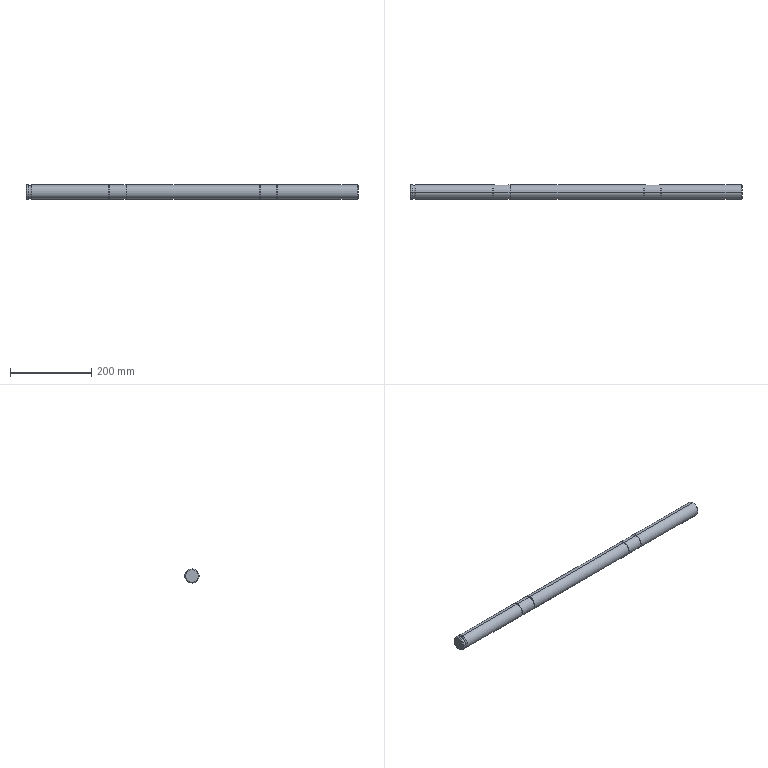Part | STEP file | IN-01-09-01 | 1 solid | 46 faces | box 816.1 x 35 x 35 mm | volume 780993 mm3 | cylinder 24 | plane 16 | cone 4 | spline 2 | commonest cylinder face diameters 35 x12 33 x8 10 x4